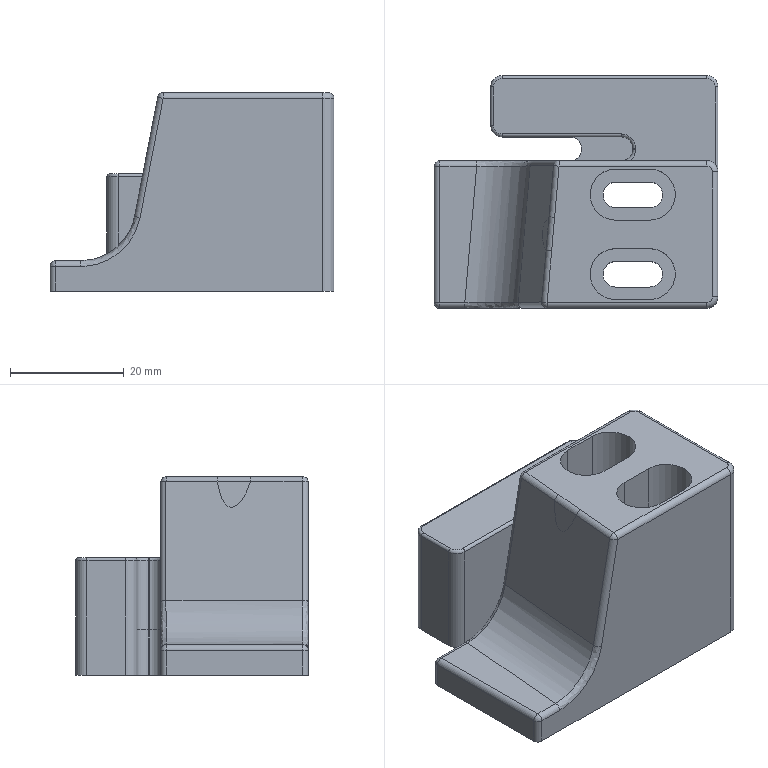NC program | NX | posted with a generic post | part box 50 x 41 x 35 mm
Whole program:
N10 G17 G21 G94 G90
(FLOOR_WALL_COPY , TOOL : D63)
N12 T01 M6
N14 G54
N16 G17 G0 G90 X-59.5 Y0. S6500 M3
N18 G43 Z30. H1
N20 Z7.
N22 G94 G1 Z4. F1250.
N24 X-56.5
N26 X56.5
N28 X59.5
N30 Z7.
N32 G0 Z30.
N34 X-59.5
N36 Z6.
N38 G1 Z3.
N40 X-56.5
N42 X56.5
N44 X59.5
N46 Z6.
N48 G0 Z30.
N50 X-59.5
N52 Z5.
N54 G1 Z2.
N56 X-56.5
N58 X56.5
N60 X59.5
N62 Z5.
N64 G0 Z30.
N66 X-59.5
N68 Z4.
N70 G1 Z1.
N72 X-56.5
N74 X56.5
N76 X59.5
N78 Z4.
N80 G0 Z30.
N82 X-59.5
N84 Z3.
N86 G1 Z0.
N88 X-56.5
N90 X56.5
N92 X59.5
N94 Z3.
N96 G0 Z30.
N98 M5
(ZLEVEL_PROFILE_1_COPY_1_COPY_COPY_COPY , TOOL : D4A45)
N100 T02 M6
N102 G54
N104 G17 G0 G90 X-13.149 Y-14.968 S9500 M3
N106 G43 Z30. H2
N108 Z0.
N110 G94 G1 Z-1. F1000.
N112 X-13.346 Y-15.591
N114 G3 X-13. Y-15.791 R0.4
N116 G1 X-7.
N118 G3 X-5.709 Y-14.5 R1.291
N120 X-7. Y-13.209 R1.291
N122 G1 X-13.
N124 G3 X-14.291 Y-14.5 R1.291
N126 X-13. Y-15.791 R1.291
N128 X-12.654 Y-15.591 R0.4
N130 G1 X-12.307 Y-14.991
N132 Z0.
N134 G0 Z30.
N136 X-13.149 Y-0.968
N138 Z0.
N140 G1 Z-1.
N142 X-13.346 Y-1.591
N144 G3 X-13. Y-1.791 R0.4
N146 G1 X-7.
N148 G3 X-5.709 Y-0.5 R1.291
N150 X-7. Y0.791 R1.291
N152 G1 X-13.
N154 G3 X-14.291 Y-0.5 R1.291
N156 X-13. Y-1.791 R1.291
N158 X-12.654 Y-1.591 R0.4
N160 G1 X-12.307 Y-0.991
N162 Z0.
N164 G0 Z30.
N166 X24.648 Y-22.181
N168 Z0.
N170 G1 Z-1.
N172 X24.346 Y-21.659
N174 G3 X24. Y-21.459 R0.4
N176 G1 X-23.
N178 G2 X-25.959 Y-18.5 R2.959
N180 G1 Y18.5
N182 G2 X-23. Y21.459 R2.959
N184 G1 X13.
N186 G2 X15.959 Y18.5 R2.959
N188 G1 Y11.7
N190 G2 X13. Y8.741 R2.959
N192 G1 X1.
N194 G3 X-0.041 Y7.7 R1.041
N196 G1 Y7.5
N198 G3 X1. Y6.459 R1.041
N200 G1 X24.
N202 G2 X25.959 Y4.5 R1.959
N204 G1 Y-19.5
N206 G2 X24. Y-21.459 R1.959
N208 G3 X23.654 Y-21.659 R0.4
N210 G1 X23.307 Y-22.259
N212 Z0.
N214 G0 Z30.
N216 M5
N218 M2